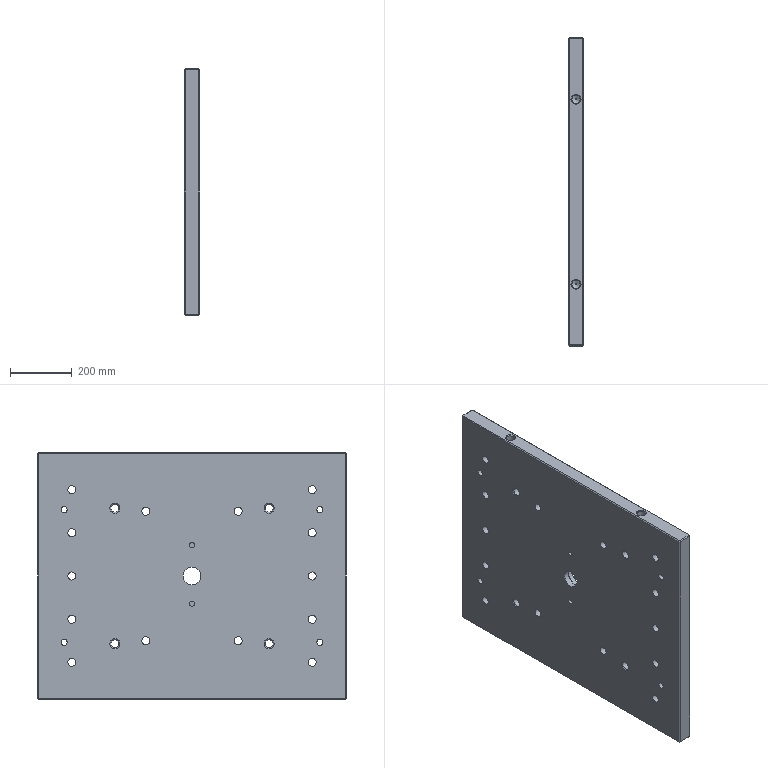Part | STEP file | solid 89 | 1 solid | 125 faces | box 50 x 1000 x 800 mm | volume 38736605 mm3 | plane 51 | cylinder 49 | cone 24 | torus 1 | commonest cylinder face diameters 26 x14 39 x14 26.5 x8 6.8 x4 20 x4 16 x2